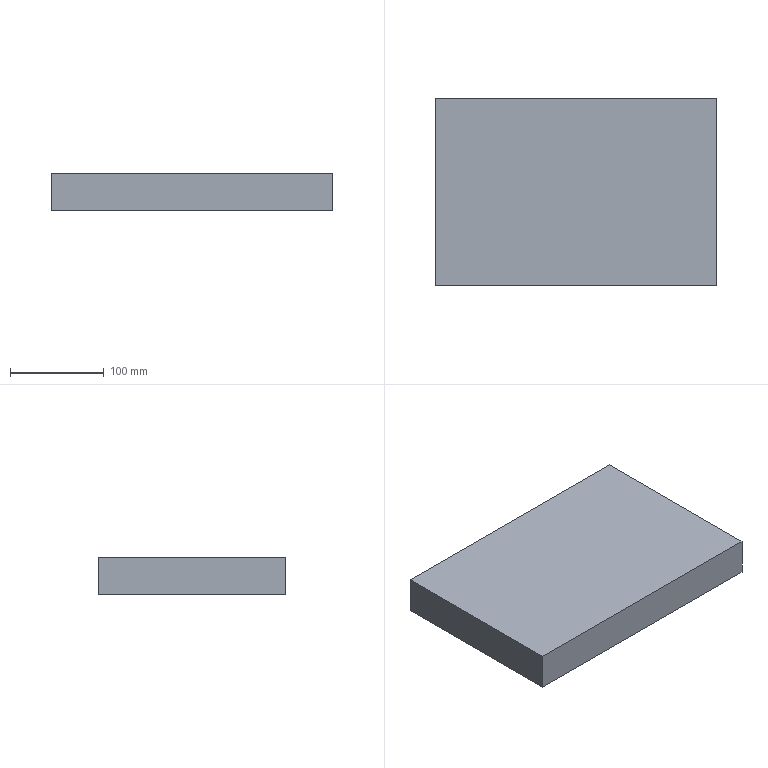Part | SolidWorks | features Extrusion 1 | 1 solid | 6 faces | box 300 x 200 x 40 mm | volume 2400000 mm3 | plane 6
STEP:
#1=CARTESIAN_POINT('',(0.,200.,0.));
#2=VERTEX_POINT('',#1);
#3=CARTESIAN_POINT('',(0.,0.,0.));
#4=VERTEX_POINT('',#3);
#5=CARTESIAN_POINT('',(0.,0.,0.));
#6=DIRECTION('',(0.,-1.,0.));
#7=VECTOR('',#6,1000.);
#8=LINE('',#5,#7);
#9=EDGE_CURVE('',#2,#4,#8,.T.);
#10=ORIENTED_EDGE('',*,*,#9,.T.);
#11=CARTESIAN_POINT('',(0.,0.,40.));
#12=VERTEX_POINT('',#11);
#13=CARTESIAN_POINT('',(0.,0.,40.));
#14=DIRECTION('',(0.,0.,-1.));
#15=VECTOR('',#14,1000.);
#16=LINE('',#13,#15);
#17=EDGE_CURVE('',#12,#4,#16,.T.);
#18=ORIENTED_EDGE('',*,*,#17,.F.);
#19=CARTESIAN_POINT('',(0.,200.,40.));
#20=VERTEX_POINT('',#19);
#21=CARTESIAN_POINT('',(0.,0.,40.));
#22=DIRECTION('',(0.,-1.,0.));
#23=VECTOR('',#22,1000.);
#24=LINE('',#21,#23);
#25=EDGE_CURVE('',#20,#12,#24,.T.);
#26=ORIENTED_EDGE('',*,*,#25,.F.);
#27=CARTESIAN_POINT('',(0.,200.,40.));
#28=DIRECTION('',(0.,0.,-1.));
#29=VECTOR('',#28,1000.);
#30=LINE('',#27,#29);
#31=EDGE_CURVE('',#20,#2,#30,.T.);
#32=ORIENTED_EDGE('',*,*,#31,.T.);
#33=EDGE_LOOP('',(#10,#18,#26,#32));
#34=FACE_OUTER_BOUND('',#33,.T.);
#35=CARTESIAN_POINT('',(0.,0.,40.));
#36=DIRECTION('',(1.,0.,0.));
#37=DIRECTION('',(0.,0.,-1.));
#38=AXIS2_PLACEMENT_3D('',#35,#36,#37);
#39=PLANE('',#38);
#40=ADVANCED_FACE('',(#34),#39,.F.);
#41=CARTESIAN_POINT('',(300.,0.,0.));
#42=VERTEX_POINT('',#41);
#43=CARTESIAN_POINT('',(0.,0.,0.));
#44=DIRECTION('',(1.,0.,0.));
#45=VECTOR('',#44,1000.);
#46=LINE('',#43,#45);
#47=EDGE_CURVE('',#4,#42,#46,.T.);
#48=ORIENTED_EDGE('',*,*,#47,.T.);
#49=CARTESIAN_POINT('',(300.,0.,40.));
#50=VERTEX_POINT('',#49);
#51=CARTESIAN_POINT('',(300.,0.,40.));
#52=DIRECTION('',(0.,0.,-1.));
#53=VECTOR('',#52,1000.);
#54=LINE('',#51,#53);
#55=EDGE_CURVE('',#50,#42,#54,.T.);
#56=ORIENTED_EDGE('',*,*,#55,.F.);
#57=CARTESIAN_POINT('',(0.,0.,40.));
#58=DIRECTION('',(1.,0.,0.));
#59=VECTOR('',#58,1000.);
#60=LINE('',#57,#59);
#61=EDGE_CURVE('',#12,#50,#60,.T.);
#62=ORIENTED_EDGE('',*,*,#61,.F.);
#63=ORIENTED_EDGE('',*,*,#17,.T.);
#64=EDGE_LOOP('',(#48,#56,#62,#63));
#65=FACE_OUTER_BOUND('',#64,.T.);
#66=CARTESIAN_POINT('',(0.,0.,40.));
#67=DIRECTION('',(0.,1.,0.));
#68=DIRECTION('',(0.,0.,1.));
#69=AXIS2_PLACEMENT_3D('',#66,#67,#68);
#70=PLANE('',#69);
#71=ADVANCED_FACE('',(#65),#70,.F.);
#72=CARTESIAN_POINT('',(300.,200.,0.));
#73=VERTEX_POINT('',#72);
#74=CARTESIAN_POINT('',(300.,0.,0.));
#75=DIRECTION('',(0.,1.,0.));
#76=VECTOR('',#75,1000.);
#77=LINE('',#74,#76);
#78=EDGE_CURVE('',#42,#73,#77,.T.);
#79=ORIENTED_EDGE('',*,*,#78,.T.);
#80=CARTESIAN_POINT('',(300.,200.,40.));
#81=VERTEX_POINT('',#80);
#82=CARTESIAN_POINT('',(300.,200.,40.));
#83=DIRECTION('',(0.,0.,-1.));
#84=VECTOR('',#83,1000.);
#85=LINE('',#82,#84);
#86=EDGE_CURVE('',#81,#73,#85,.T.);
#87=ORIENTED_EDGE('',*,*,#86,.F.);
#88=CARTESIAN_POINT('',(300.,0.,40.));
#89=DIRECTION('',(0.,1.,0.));
#90=VECTOR('',#89,1000.);
#91=LINE('',#88,#90);
#92=EDGE_CURVE('',#50,#81,#91,.T.);
#93=ORIENTED_EDGE('',*,*,#92,.F.);
#94=ORIENTED_EDGE('',*,*,#55,.T.);
#95=EDGE_LOOP('',(#79,#87,#93,#94));
#96=FACE_OUTER_BOUND('',#95,.T.);
#97=CARTESIAN_POINT('',(300.,0.,40.));
#98=DIRECTION('',(-1.,0.,0.));
#99=DIRECTION('',(0.,0.,1.));
#100=AXIS2_PLACEMENT_3D('',#97,#98,#99);
#101=PLANE('',#100);
#102=ADVANCED_FACE('',(#96),#101,.F.);
#103=CARTESIAN_POINT('',(0.,200.,0.));
#104=DIRECTION('',(-1.,0.,0.));
#105=VECTOR('',#104,1000.);
#106=LINE('',#103,#105);
#107=EDGE_CURVE('',#73,#2,#106,.T.);
#108=ORIENTED_EDGE('',*,*,#107,.T.);
#109=ORIENTED_EDGE('',*,*,#31,.F.);
#110=CARTESIAN_POINT('',(0.,200.,40.));
#111=DIRECTION('',(-1.,0.,0.));
#112=VECTOR('',#111,1000.);
#113=LINE('',#110,#112);
#114=EDGE_CURVE('',#81,#20,#113,.T.);
#115=ORIENTED_EDGE('',*,*,#114,.F.);
#116=ORIENTED_EDGE('',*,*,#86,.T.);
#117=EDGE_LOOP('',(#108,#109,#115,#116));
#118=FACE_OUTER_BOUND('',#117,.T.);
#119=CARTESIAN_POINT('',(0.,200.,40.));
#120=DIRECTION('',(0.,-1.,0.));
#121=DIRECTION('',(0.,0.,-1.));
#122=AXIS2_PLACEMENT_3D('',#119,#120,#121);
#123=PLANE('',#122);
#124=ADVANCED_FACE('',(#118),#123,.F.);
#125=ORIENTED_EDGE('',*,*,#25,.T.);
#126=ORIENTED_EDGE('',*,*,#61,.T.);
#127=ORIENTED_EDGE('',*,*,#92,.T.);
#128=ORIENTED_EDGE('',*,*,#114,.T.);
#129=EDGE_LOOP('',(#125,#126,#127,#128));
#130=FACE_OUTER_BOUND('',#129,.T.);
#131=CARTESIAN_POINT('',(0.,0.,40.));
#132=DIRECTION('',(0.,0.,-1.));
#133=DIRECTION('',(-1.,0.,0.));
#134=AXIS2_PLACEMENT_3D('',#131,#132,#133);
#135=PLANE('',#134);
#136=ADVANCED_FACE('',(#130),#135,.F.);
#137=ORIENTED_EDGE('',*,*,#9,.F.);
#138=ORIENTED_EDGE('',*,*,#107,.F.);
#139=ORIENTED_EDGE('',*,*,#78,.F.);
#140=ORIENTED_EDGE('',*,*,#47,.F.);
#141=EDGE_LOOP('',(#137,#138,#139,#140));
#142=FACE_OUTER_BOUND('',#141,.T.);
#143=CARTESIAN_POINT('',(0.,0.,0.));
#144=DIRECTION('',(0.,0.,-1.));
#145=DIRECTION('',(-1.,0.,0.));
#146=AXIS2_PLACEMENT_3D('',#143,#144,#145);
#147=PLANE('',#146);
#148=ADVANCED_FACE('',(#142),#147,.T.);
#149=CLOSED_SHELL('',(#40,#71,#102,#124,#136,#148));
#150=MANIFOLD_SOLID_BREP('',#149);
#151=CARTESIAN_POINT('',(0.,0.,0.));
#152=DIRECTION('',(0.,0.,1.));
#153=DIRECTION('',(1.,0.,0.));
#154=AXIS2_PLACEMENT_3D('',#151,#152,#153);
#155=(LENGTH_UNIT()NAMED_UNIT(*)SI_UNIT(.MILLI.,.METRE.));
#156=UNCERTAINTY_MEASURE_WITH_UNIT(LENGTH_MEASURE(0.00001),#155,'','');
#157=(NAMED_UNIT(*)PLANE_ANGLE_UNIT()SI_UNIT($,.RADIAN.));
#158=(NAMED_UNIT(*)SI_UNIT($,.STERADIAN.)SOLID_ANGLE_UNIT());
#159=(GEOMETRIC_REPRESENTATION_CONTEXT(3)GLOBAL_UNCERTAINTY_ASSIGNED_CONTEXT((#156))GLOBAL_UNIT_ASSIGNED_CONTEXT((#155,#157,#158))REPRESENTATION_CONTEXT('',''));
#160=ADVANCED_BREP_SHAPE_REPRESENTATION('',(#150,#154),#159);